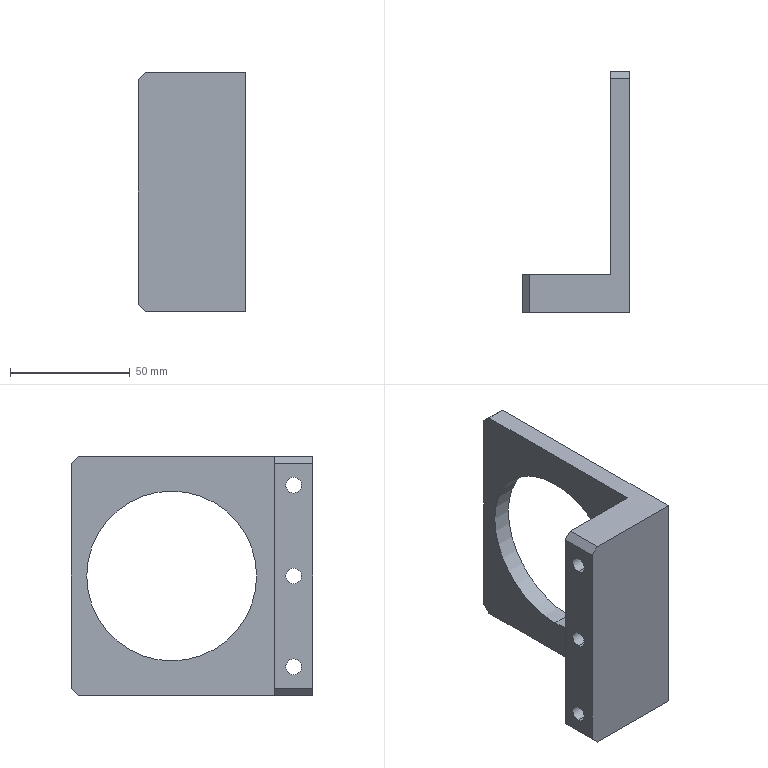Part | SolidWorks | features 3DProfileFeature 1, Chamfer 1, Extrusion 1, HoleWzd 1, ICE 1 | 1 solid | 29 faces | box 45 x 101 x 100 mm | volume 97106 mm3 | plane 15 | cylinder 14 | commonest cylinder face diameters 6.6 x6 11 x6 71 x2
STEP:
#1=CARTESIAN_POINT('',(-35.,8.,9.121));
#2=VERTEX_POINT('',#1);
#3=CARTESIAN_POINT('',(-35.,8.,-1.879));
#4=VERTEX_POINT('',#3);
#5=CARTESIAN_POINT('',(-35.,8.,3.621));
#6=DIRECTION('',(1.,0.,0.));
#7=DIRECTION('',(0.,0.,-1.));
#8=AXIS2_PLACEMENT_3D('',#5,#6,#7);
#9=CIRCLE('',#8,5.5);
#10=EDGE_CURVE('',#2,#4,#9,.T.);
#11=ORIENTED_EDGE('',*,*,#10,.F.);
#12=CARTESIAN_POINT('',(0.,8.,9.121));
#13=VERTEX_POINT('',#12);
#14=CARTESIAN_POINT('',(0.,8.,9.121));
#15=DIRECTION('',(1.,0.,0.));
#16=VECTOR('',#15,1000.);
#17=LINE('',#14,#16);
#18=EDGE_CURVE('',#2,#13,#17,.T.);
#19=ORIENTED_EDGE('',*,*,#18,.T.);
#20=CARTESIAN_POINT('',(0.,8.,-1.879));
#21=VERTEX_POINT('',#20);
#22=CARTESIAN_POINT('',(0.,8.,3.621));
#23=DIRECTION('',(1.,0.,0.));
#24=DIRECTION('',(0.,0.,-1.));
#25=AXIS2_PLACEMENT_3D('',#22,#23,#24);
#26=CIRCLE('',#25,5.5);
#27=EDGE_CURVE('',#13,#21,#26,.T.);
#28=ORIENTED_EDGE('',*,*,#27,.T.);
#29=CARTESIAN_POINT('',(0.,8.,-1.879));
#30=DIRECTION('',(1.,0.,0.));
#31=VECTOR('',#30,1000.);
#32=LINE('',#29,#31);
#33=EDGE_CURVE('',#4,#21,#32,.T.);
#34=ORIENTED_EDGE('',*,*,#33,.F.);
#35=EDGE_LOOP('',(#11,#19,#28,#34));
#36=FACE_OUTER_BOUND('',#35,.T.);
#37=CARTESIAN_POINT('',(0.,8.,3.621));
#38=DIRECTION('',(1.,0.,0.));
#39=DIRECTION('',(0.,0.,-1.));
#40=AXIS2_PLACEMENT_3D('',#37,#38,#39);
#41=CYLINDRICAL_SURFACE('',#40,5.5);
#42=ADVANCED_FACE('',(#36),#41,.F.);
#43=CARTESIAN_POINT('',(-45.,8.,6.921));
#44=VERTEX_POINT('',#43);
#45=CARTESIAN_POINT('',(-45.,8.,0.3205));
#46=VERTEX_POINT('',#45);
#47=CARTESIAN_POINT('',(-45.,8.,3.621));
#48=DIRECTION('',(1.,0.,0.));
#49=DIRECTION('',(0.,0.,-1.));
#50=AXIS2_PLACEMENT_3D('',#47,#48,#49);
#51=CIRCLE('',#50,3.3);
#52=EDGE_CURVE('',#44,#46,#51,.T.);
#53=ORIENTED_EDGE('',*,*,#52,.F.);
#54=CARTESIAN_POINT('',(-35.,8.,6.921));
#55=VERTEX_POINT('',#54);
#56=CARTESIAN_POINT('',(0.,8.,6.921));
#57=DIRECTION('',(1.,0.,0.));
#58=VECTOR('',#57,1000.);
#59=LINE('',#56,#58);
#60=EDGE_CURVE('',#44,#55,#59,.T.);
#61=ORIENTED_EDGE('',*,*,#60,.T.);
#62=CARTESIAN_POINT('',(-35.,8.,0.3205));
#63=VERTEX_POINT('',#62);
#64=CARTESIAN_POINT('',(-35.,8.,3.621));
#65=DIRECTION('',(1.,0.,0.));
#66=DIRECTION('',(0.,0.,-1.));
#67=AXIS2_PLACEMENT_3D('',#64,#65,#66);
#68=CIRCLE('',#67,3.3);
#69=EDGE_CURVE('',#55,#63,#68,.T.);
#70=ORIENTED_EDGE('',*,*,#69,.T.);
#71=CARTESIAN_POINT('',(0.,8.,0.3205));
#72=DIRECTION('',(1.,0.,0.));
#73=VECTOR('',#72,1000.);
#74=LINE('',#71,#73);
#75=EDGE_CURVE('',#46,#63,#74,.T.);
#76=ORIENTED_EDGE('',*,*,#75,.F.);
#77=EDGE_LOOP('',(#53,#61,#70,#76));
#78=FACE_OUTER_BOUND('',#77,.T.);
#79=CARTESIAN_POINT('',(0.,8.,3.621));
#80=DIRECTION('',(1.,0.,0.));
#81=DIRECTION('',(0.,0.,-1.));
#82=AXIS2_PLACEMENT_3D('',#79,#80,#81);
#83=CYLINDRICAL_SURFACE('',#82,3.3);
#84=ADVANCED_FACE('',(#78),#83,.F.);
#85=CARTESIAN_POINT('',(-35.,8.,-28.879));
#86=VERTEX_POINT('',#85);
#87=CARTESIAN_POINT('',(-35.,8.,-39.879));
#88=VERTEX_POINT('',#87);
#89=CARTESIAN_POINT('',(-35.,8.,-34.379));
#90=DIRECTION('',(1.,0.,0.));
#91=DIRECTION('',(0.,0.,-1.));
#92=AXIS2_PLACEMENT_3D('',#89,#90,#91);
#93=CIRCLE('',#92,5.5);
#94=EDGE_CURVE('',#86,#88,#93,.T.);
#95=ORIENTED_EDGE('',*,*,#94,.F.);
#96=CARTESIAN_POINT('',(0.,8.,-28.879));
#97=VERTEX_POINT('',#96);
#98=CARTESIAN_POINT('',(0.,8.,-28.879));
#99=DIRECTION('',(1.,0.,0.));
#100=VECTOR('',#99,1000.);
#101=LINE('',#98,#100);
#102=EDGE_CURVE('',#86,#97,#101,.T.);
#103=ORIENTED_EDGE('',*,*,#102,.T.);
#104=CARTESIAN_POINT('',(0.,8.,-39.879));
#105=VERTEX_POINT('',#104);
#106=CARTESIAN_POINT('',(0.,8.,-34.379));
#107=DIRECTION('',(1.,0.,0.));
#108=DIRECTION('',(0.,0.,-1.));
#109=AXIS2_PLACEMENT_3D('',#106,#107,#108);
#110=CIRCLE('',#109,5.5);
#111=EDGE_CURVE('',#97,#105,#110,.T.);
#112=ORIENTED_EDGE('',*,*,#111,.T.);
#113=CARTESIAN_POINT('',(0.,8.,-39.879));
#114=DIRECTION('',(1.,0.,0.));
#115=VECTOR('',#114,1000.);
#116=LINE('',#113,#115);
#117=EDGE_CURVE('',#88,#105,#116,.T.);
#118=ORIENTED_EDGE('',*,*,#117,.F.);
#119=EDGE_LOOP('',(#95,#103,#112,#118));
#120=FACE_OUTER_BOUND('',#119,.T.);
#121=CARTESIAN_POINT('',(0.,8.,-34.379));
#122=DIRECTION('',(1.,0.,0.));
#123=DIRECTION('',(0.,0.,-1.));
#124=AXIS2_PLACEMENT_3D('',#121,#122,#123);
#125=CYLINDRICAL_SURFACE('',#124,5.5);
#126=ADVANCED_FACE('',(#120),#125,.F.);
#127=CARTESIAN_POINT('',(-45.,8.,-31.079));
#128=VERTEX_POINT('',#127);
#129=CARTESIAN_POINT('',(-45.,8.,-37.679));
#130=VERTEX_POINT('',#129);
#131=CARTESIAN_POINT('',(-45.,8.,-34.379));
#132=DIRECTION('',(1.,0.,0.));
#133=DIRECTION('',(0.,0.,-1.));
#134=AXIS2_PLACEMENT_3D('',#131,#132,#133);
#135=CIRCLE('',#134,3.3);
#136=EDGE_CURVE('',#128,#130,#135,.T.);
#137=ORIENTED_EDGE('',*,*,#136,.F.);
#138=CARTESIAN_POINT('',(-35.,8.,-31.079));
#139=VERTEX_POINT('',#138);
#140=CARTESIAN_POINT('',(0.,8.,-31.079));
#141=DIRECTION('',(1.,0.,0.));
#142=VECTOR('',#141,1000.);
#143=LINE('',#140,#142);
#144=EDGE_CURVE('',#128,#139,#143,.T.);
#145=ORIENTED_EDGE('',*,*,#144,.T.);
#146=CARTESIAN_POINT('',(-35.,8.,-37.679));
#147=VERTEX_POINT('',#146);
#148=CARTESIAN_POINT('',(-35.,8.,-34.379));
#149=DIRECTION('',(1.,0.,0.));
#150=DIRECTION('',(0.,0.,-1.));
#151=AXIS2_PLACEMENT_3D('',#148,#149,#150);
#152=CIRCLE('',#151,3.3);
#153=EDGE_CURVE('',#139,#147,#152,.T.);
#154=ORIENTED_EDGE('',*,*,#153,.T.);
#155=CARTESIAN_POINT('',(0.,8.,-37.679));
#156=DIRECTION('',(1.,0.,0.));
#157=VECTOR('',#156,1000.);
#158=LINE('',#155,#157);
#159=EDGE_CURVE('',#130,#147,#158,.T.);
#160=ORIENTED_EDGE('',*,*,#159,.F.);
#161=EDGE_LOOP('',(#137,#145,#154,#160));
#162=FACE_OUTER_BOUND('',#161,.T.);
#163=CARTESIAN_POINT('',(0.,8.,-34.379));
#164=DIRECTION('',(1.,0.,0.));
#165=DIRECTION('',(0.,0.,-1.));
#166=AXIS2_PLACEMENT_3D('',#163,#164,#165);
#167=CYLINDRICAL_SURFACE('',#166,3.3);
#168=ADVANCED_FACE('',(#162),#167,.F.);
#169=CARTESIAN_POINT('',(-35.,8.,-66.879));
#170=VERTEX_POINT('',#169);
#171=CARTESIAN_POINT('',(-35.,8.,-77.879));
#172=VERTEX_POINT('',#171);
#173=CARTESIAN_POINT('',(-35.,8.,-72.379));
#174=DIRECTION('',(1.,0.,0.));
#175=DIRECTION('',(0.,0.,-1.));
#176=AXIS2_PLACEMENT_3D('',#173,#174,#175);
#177=CIRCLE('',#176,5.5);
#178=EDGE_CURVE('',#170,#172,#177,.T.);
#179=ORIENTED_EDGE('',*,*,#178,.F.);
#180=CARTESIAN_POINT('',(0.,8.,-66.879));
#181=VERTEX_POINT('',#180);
#182=CARTESIAN_POINT('',(0.,8.,-66.879));
#183=DIRECTION('',(1.,0.,0.));
#184=VECTOR('',#183,1000.);
#185=LINE('',#182,#184);
#186=EDGE_CURVE('',#170,#181,#185,.T.);
#187=ORIENTED_EDGE('',*,*,#186,.T.);
#188=CARTESIAN_POINT('',(0.,8.,-77.879));
#189=VERTEX_POINT('',#188);
#190=CARTESIAN_POINT('',(0.,8.,-72.379));
#191=DIRECTION('',(1.,0.,0.));
#192=DIRECTION('',(0.,0.,-1.));
#193=AXIS2_PLACEMENT_3D('',#190,#191,#192);
#194=CIRCLE('',#193,5.5);
#195=EDGE_CURVE('',#181,#189,#194,.T.);
#196=ORIENTED_EDGE('',*,*,#195,.T.);
#197=CARTESIAN_POINT('',(0.,8.,-77.879));
#198=DIRECTION('',(1.,0.,0.));
#199=VECTOR('',#198,1000.);
#200=LINE('',#197,#199);
#201=EDGE_CURVE('',#172,#189,#200,.T.);
#202=ORIENTED_EDGE('',*,*,#201,.F.);
#203=EDGE_LOOP('',(#179,#187,#196,#202));
#204=FACE_OUTER_BOUND('',#203,.T.);
#205=CARTESIAN_POINT('',(0.,8.,-72.379));
#206=DIRECTION('',(1.,0.,0.));
#207=DIRECTION('',(0.,0.,-1.));
#208=AXIS2_PLACEMENT_3D('',#205,#206,#207);
#209=CYLINDRICAL_SURFACE('',#208,5.5);
#210=ADVANCED_FACE('',(#204),#209,.F.);
#211=CARTESIAN_POINT('',(-45.,8.,-69.079));
#212=VERTEX_POINT('',#211);
#213=CARTESIAN_POINT('',(-45.,8.,-75.679));
#214=VERTEX_POINT('',#213);
#215=CARTESIAN_POINT('',(-45.,8.,-72.379));
#216=DIRECTION('',(1.,0.,0.));
#217=DIRECTION('',(0.,0.,-1.));
#218=AXIS2_PLACEMENT_3D('',#215,#216,#217);
#219=CIRCLE('',#218,3.3);
#220=EDGE_CURVE('',#212,#214,#219,.T.);
#221=ORIENTED_EDGE('',*,*,#220,.F.);
#222=CARTESIAN_POINT('',(-35.,8.,-69.079));
#223=VERTEX_POINT('',#222);
#224=CARTESIAN_POINT('',(0.,8.,-69.079));
#225=DIRECTION('',(1.,0.,0.));
#226=VECTOR('',#225,1000.);
#227=LINE('',#224,#226);
#228=EDGE_CURVE('',#212,#223,#227,.T.);
#229=ORIENTED_EDGE('',*,*,#228,.T.);
#230=CARTESIAN_POINT('',(-35.,8.,-75.679));
#231=VERTEX_POINT('',#230);
#232=CARTESIAN_POINT('',(-35.,8.,-72.379));
#233=DIRECTION('',(1.,0.,0.));
#234=DIRECTION('',(0.,0.,-1.));
#235=AXIS2_PLACEMENT_3D('',#232,#233,#234);
#236=CIRCLE('',#235,3.3);
#237=EDGE_CURVE('',#223,#231,#236,.T.);
#238=ORIENTED_EDGE('',*,*,#237,.T.);
#239=CARTESIAN_POINT('',(0.,8.,-75.679));
#240=DIRECTION('',(1.,0.,0.));
#241=VECTOR('',#240,1000.);
#242=LINE('',#239,#241);
#243=EDGE_CURVE('',#214,#231,#242,.T.);
#244=ORIENTED_EDGE('',*,*,#243,.F.);
#245=EDGE_LOOP('',(#221,#229,#238,#244));
#246=FACE_OUTER_BOUND('',#245,.T.);
#247=CARTESIAN_POINT('',(0.,8.,-72.379));
#248=DIRECTION('',(1.,0.,0.));
#249=DIRECTION('',(0.,0.,-1.));
#250=AXIS2_PLACEMENT_3D('',#247,#248,#249);
#251=CYLINDRICAL_SURFACE('',#250,3.3);
#252=ADVANCED_FACE('',(#246),#251,.F.);
#253=CARTESIAN_POINT('',(0.,59.,1.121));
#254=VERTEX_POINT('',#253);
#255=CARTESIAN_POINT('',(0.,59.,-69.879));
#256=VERTEX_POINT('',#255);
#257=CARTESIAN_POINT('',(0.,59.,-34.379));
#258=DIRECTION('',(1.,0.,0.));
#259=DIRECTION('',(0.,0.,1.));
#260=AXIS2_PLACEMENT_3D('',#257,#258,#259);
#261=CIRCLE('',#260,35.5);
#262=EDGE_CURVE('',#254,#256,#261,.T.);
#263=ORIENTED_EDGE('',*,*,#262,.T.);
#264=CARTESIAN_POINT('',(-8.,59.,-69.879));
#265=VERTEX_POINT('',#264);
#266=CARTESIAN_POINT('',(0.001,59.,-69.879));
#267=DIRECTION('',(-1.,0.,0.));
#268=VECTOR('',#267,1000.);
#269=LINE('',#266,#268);
#270=EDGE_CURVE('',#256,#265,#269,.T.);
#271=ORIENTED_EDGE('',*,*,#270,.T.);
#272=CARTESIAN_POINT('',(-8.,59.,1.121));
#273=VERTEX_POINT('',#272);
#274=CARTESIAN_POINT('',(-8.,59.,-34.379));
#275=DIRECTION('',(-1.,0.,0.));
#276=DIRECTION('',(0.,0.,1.));
#277=AXIS2_PLACEMENT_3D('',#274,#275,#276);
#278=CIRCLE('',#277,35.5);
#279=EDGE_CURVE('',#265,#273,#278,.T.);
#280=ORIENTED_EDGE('',*,*,#279,.T.);
#281=CARTESIAN_POINT('',(0.001,59.,1.121));
#282=DIRECTION('',(-1.,0.,0.));
#283=VECTOR('',#282,1000.);
#284=LINE('',#281,#283);
#285=EDGE_CURVE('',#254,#273,#284,.T.);
#286=ORIENTED_EDGE('',*,*,#285,.F.);
#287=EDGE_LOOP('',(#263,#271,#280,#286));
#288=FACE_OUTER_BOUND('',#287,.T.);
#289=CARTESIAN_POINT('',(0.001,59.,-34.379));
#290=DIRECTION('',(-1.,0.,0.));
#291=DIRECTION('',(0.,0.,1.));
#292=AXIS2_PLACEMENT_3D('',#289,#290,#291);
#293=CYLINDRICAL_SURFACE('',#292,35.5);
#294=ADVANCED_FACE('',(#288),#293,.F.);
#295=CARTESIAN_POINT('',(0.,8.,-34.379));
#296=DIRECTION('',(1.,0.,0.));
#297=DIRECTION('',(0.,0.,-1.));
#298=AXIS2_PLACEMENT_3D('',#295,#296,#297);
#299=CIRCLE('',#298,5.5);
#300=EDGE_CURVE('',#105,#97,#299,.T.);
#301=ORIENTED_EDGE('',*,*,#300,.F.);
#302=ORIENTED_EDGE('',*,*,#111,.F.);
#303=EDGE_LOOP('',(#301,#302));
#304=FACE_BOUND('',#303,.T.);
#305=ORIENTED_EDGE('',*,*,#262,.F.);
#306=CARTESIAN_POINT('',(0.,59.,-34.379));
#307=DIRECTION('',(1.,0.,0.));
#308=DIRECTION('',(0.,0.,1.));
#309=AXIS2_PLACEMENT_3D('',#306,#307,#308);
#310=CIRCLE('',#309,35.5);
#311=EDGE_CURVE('',#256,#254,#310,.T.);
#312=ORIENTED_EDGE('',*,*,#311,.F.);
#313=EDGE_LOOP('',(#305,#312));
#314=FACE_BOUND('',#313,.T.);
#315=CARTESIAN_POINT('',(0.,101.,12.621));
#316=VERTEX_POINT('',#315);
#317=CARTESIAN_POINT('',(0.,101.,-81.379));
#318=VERTEX_POINT('',#317);
#319=CARTESIAN_POINT('',(0.,101.,15.621));
#320=DIRECTION('',(0.,0.,-1.));
#321=VECTOR('',#320,1000.);
#322=LINE('',#319,#321);
#323=EDGE_CURVE('',#316,#318,#322,.T.);
#324=ORIENTED_EDGE('',*,*,#323,.F.);
#325=CARTESIAN_POINT('',(0.,98.,15.621));
#326=VERTEX_POINT('',#325);
#327=CARTESIAN_POINT('',(0.,98.,15.621));
#328=DIRECTION('',(0.,-0.7071,0.7071));
#329=VECTOR('',#328,1000.);
#330=LINE('',#327,#329);
#331=EDGE_CURVE('',#316,#326,#330,.T.);
#332=ORIENTED_EDGE('',*,*,#331,.T.);
#333=CARTESIAN_POINT('',(0.,0.,15.621));
#334=VERTEX_POINT('',#333);
#335=CARTESIAN_POINT('',(0.,101.,15.621));
#336=DIRECTION('',(0.,1.,0.));
#337=VECTOR('',#336,1000.);
#338=LINE('',#335,#337);
#339=EDGE_CURVE('',#334,#326,#338,.T.);
#340=ORIENTED_EDGE('',*,*,#339,.F.);
#341=CARTESIAN_POINT('',(0.,0.,-84.379));
#342=VERTEX_POINT('',#341);
#343=CARTESIAN_POINT('',(0.,0.,15.621));
#344=DIRECTION('',(0.,0.,-1.));
#345=VECTOR('',#344,1000.);
#346=LINE('',#343,#345);
#347=EDGE_CURVE('',#334,#342,#346,.T.);
#348=ORIENTED_EDGE('',*,*,#347,.T.);
#349=CARTESIAN_POINT('',(0.,98.,-84.379));
#350=VERTEX_POINT('',#349);
#351=CARTESIAN_POINT('',(0.,101.,-84.379));
#352=DIRECTION('',(0.,1.,0.));
#353=VECTOR('',#352,1000.);
#354=LINE('',#351,#353);
#355=EDGE_CURVE('',#342,#350,#354,.T.);
#356=ORIENTED_EDGE('',*,*,#355,.T.);
#357=CARTESIAN_POINT('',(0.,101.,-81.379));
#358=DIRECTION('',(0.,0.7071,0.7071));
#359=VECTOR('',#358,1000.);
#360=LINE('',#357,#359);
#361=EDGE_CURVE('',#350,#318,#360,.T.);
#362=ORIENTED_EDGE('',*,*,#361,.T.);
#363=EDGE_LOOP('',(#324,#332,#340,#348,#356,#362));
#364=FACE_OUTER_BOUND('',#363,.T.);
#365=CARTESIAN_POINT('',(0.,8.,-72.379));
#366=DIRECTION('',(1.,0.,0.));
#367=DIRECTION('',(0.,0.,-1.));
#368=AXIS2_PLACEMENT_3D('',#365,#366,#367);
#369=CIRCLE('',#368,5.5);
#370=EDGE_CURVE('',#189,#181,#369,.T.);
#371=ORIENTED_EDGE('',*,*,#370,.F.);
#372=ORIENTED_EDGE('',*,*,#195,.F.);
#373=EDGE_LOOP('',(#371,#372));
#374=FACE_BOUND('',#373,.T.);
#375=CARTESIAN_POINT('',(0.,8.,3.621));
#376=DIRECTION('',(1.,0.,0.));
#377=DIRECTION('',(0.,0.,-1.));
#378=AXIS2_PLACEMENT_3D('',#375,#376,#377);
#379=CIRCLE('',#378,5.5);
#380=EDGE_CURVE('',#21,#13,#379,.T.);
#381=ORIENTED_EDGE('',*,*,#380,.F.);
#382=ORIENTED_EDGE('',*,*,#27,.F.);
#383=EDGE_LOOP('',(#381,#382));
#384=FACE_BOUND('',#383,.T.);
#385=CARTESIAN_POINT('',(0.,101.,15.621));
#386=DIRECTION('',(-1.,0.,0.));
#387=DIRECTION('',(0.,0.,1.));
#388=AXIS2_PLACEMENT_3D('',#385,#386,#387);
#389=PLANE('',#388);
#390=ADVANCED_FACE('',(#304,#314,#364,#374,#384),#389,.F.);
#391=CARTESIAN_POINT('',(-8.,101.,12.621));
#392=VERTEX_POINT('',#391);
#393=CARTESIAN_POINT('',(-8.,101.,-81.379));
#394=VERTEX_POINT('',#393);
#395=CARTESIAN_POINT('',(-8.,101.,15.621));
#396=DIRECTION('',(0.,0.,-1.));
#397=VECTOR('',#396,1000.);
#398=LINE('',#395,#397);
#399=EDGE_CURVE('',#392,#394,#398,.T.);
#400=ORIENTED_EDGE('',*,*,#399,.F.);
#401=CARTESIAN_POINT('',(-8.,101.,12.621));
#402=DIRECTION('',(1.,0.,0.));
#403=VECTOR('',#402,1000.);
#404=LINE('',#401,#403);
#405=EDGE_CURVE('',#392,#316,#404,.T.);
#406=ORIENTED_EDGE('',*,*,#405,.T.);
#407=ORIENTED_EDGE('',*,*,#323,.T.);
#408=CARTESIAN_POINT('',(-8.,101.,-81.379));
#409=DIRECTION('',(-1.,0.,0.));
#410=VECTOR('',#409,1000.);
#411=LINE('',#408,#410);
#412=EDGE_CURVE('',#318,#394,#411,.T.);
#413=ORIENTED_EDGE('',*,*,#412,.T.);
#414=EDGE_LOOP('',(#400,#406,#407,#413));
#415=FACE_OUTER_BOUND('',#414,.T.);
#416=CARTESIAN_POINT('',(-8.,101.,15.621));
#417=DIRECTION('',(0.,-1.,0.));
#418=DIRECTION('',(0.,0.,-1.));
#419=AXIS2_PLACEMENT_3D('',#416,#417,#418);
#420=PLANE('',#419);
#421=ADVANCED_FACE('',(#415),#420,.F.);
#422=CARTESIAN_POINT('',(-8.,59.,-34.379));
#423=DIRECTION('',(-1.,0.,0.));
#424=DIRECTION('',(0.,0.,1.));
#425=AXIS2_PLACEMENT_3D('',#422,#423,#424);
#426=CIRCLE('',#425,35.5);
#427=EDGE_CURVE('',#273,#265,#426,.T.);
#428=ORIENTED_EDGE('',*,*,#427,.F.);
#429=ORIENTED_EDGE('',*,*,#279,.F.);
#430=EDGE_LOOP('',(#428,#429));
#431=FACE_BOUND('',#430,.T.);
#432=CARTESIAN_POINT('',(-8.,98.,15.621));
#433=VERTEX_POINT('',#432);
#434=CARTESIAN_POINT('',(-8.,16.,15.621));
#435=VERTEX_POINT('',#434);
#436=CARTESIAN_POINT('',(-8.,16.,15.621));
#437=DIRECTION('',(0.,-1.,0.));
#438=VECTOR('',#437,1000.);
#439=LINE('',#436,#438);
#440=EDGE_CURVE('',#433,#435,#439,.T.);
#441=ORIENTED_EDGE('',*,*,#440,.F.);
#442=CARTESIAN_POINT('',(-8.,98.,15.621));
#443=DIRECTION('',(0.,0.7071,-0.7071));
#444=VECTOR('',#443,1000.);
#445=LINE('',#442,#444);
#446=EDGE_CURVE('',#433,#392,#445,.T.);
#447=ORIENTED_EDGE('',*,*,#446,.T.);
#448=ORIENTED_EDGE('',*,*,#399,.T.);
#449=CARTESIAN_POINT('',(-8.,98.,-84.379));
#450=VERTEX_POINT('',#449);
#451=CARTESIAN_POINT('',(-8.,101.,-81.379));
#452=DIRECTION('',(0.,-0.7071,-0.7071));
#453=VECTOR('',#452,1000.);
#454=LINE('',#451,#453);
#455=EDGE_CURVE('',#394,#450,#454,.T.);
#456=ORIENTED_EDGE('',*,*,#455,.T.);
#457=CARTESIAN_POINT('',(-8.,16.,-84.379));
#458=VERTEX_POINT('',#457);
#459=CARTESIAN_POINT('',(-8.,16.,-84.379));
#460=DIRECTION('',(0.,-1.,0.));
#461=VECTOR('',#460,1000.);
#462=LINE('',#459,#461);
#463=EDGE_CURVE('',#450,#458,#462,.T.);
#464=ORIENTED_EDGE('',*,*,#463,.T.);
#465=CARTESIAN_POINT('',(-8.,16.,15.621));
#466=DIRECTION('',(0.,0.,-1.));
#467=VECTOR('',#466,1000.);
#468=LINE('',#465,#467);
#469=EDGE_CURVE('',#435,#458,#468,.T.);
#470=ORIENTED_EDGE('',*,*,#469,.F.);
#471=EDGE_LOOP('',(#441,#447,#448,#456,#464,#470));
#472=FACE_OUTER_BOUND('',#471,.T.);
#473=CARTESIAN_POINT('',(-8.,16.,15.621));
#474=DIRECTION('',(1.,0.,0.));
#475=DIRECTION('',(0.,0.,-1.));
#476=AXIS2_PLACEMENT_3D('',#473,#474,#475);
#477=PLANE('',#476);
#478=ADVANCED_FACE('',(#431,#472),#477,.F.);
#479=CARTESIAN_POINT('',(-42.,16.,-84.379));
#480=VERTEX_POINT('',#479);
#481=CARTESIAN_POINT('',(-45.,16.,-84.379));
#482=DIRECTION('',(-1.,0.,0.));
#483=VECTOR('',#482,1000.);
#484=LINE('',#481,#483);
#485=EDGE_CURVE('',#458,#480,#484,.T.);
#486=ORIENTED_EDGE('',*,*,#485,.T.);
#487=CARTESIAN_POINT('',(-45.,16.,-81.379));
#488=VERTEX_POINT('',#487);
#489=CARTESIAN_POINT('',(-45.,16.,-81.379));
#490=DIRECTION('',(-0.7071,0.,0.7071));
#491=VECTOR('',#490,1000.);
#492=LINE('',#489,#491);
#493=EDGE_CURVE('',#480,#488,#492,.T.);
#494=ORIENTED_EDGE('',*,*,#493,.T.);
#495=CARTESIAN_POINT('',(-45.,16.,12.621));
#496=VERTEX_POINT('',#495);
#497=CARTESIAN_POINT('',(-45.,16.,15.621));
#498=DIRECTION('',(0.,0.,-1.));
#499=VECTOR('',#498,1000.);
#500=LINE('',#497,#499);
#501=EDGE_CURVE('',#496,#488,#500,.T.);
#502=ORIENTED_EDGE('',*,*,#501,.F.);
#503=CARTESIAN_POINT('',(-42.,16.,15.621));
#504=VERTEX_POINT('',#503);
#505=CARTESIAN_POINT('',(-42.,16.,15.621));
#506=DIRECTION('',(0.7071,0.,0.7071));
#507=VECTOR('',#506,1000.);
#508=LINE('',#505,#507);
#509=EDGE_CURVE('',#496,#504,#508,.T.);
#510=ORIENTED_EDGE('',*,*,#509,.T.);
#511=CARTESIAN_POINT('',(-45.,16.,15.621));
#512=DIRECTION('',(-1.,0.,0.));
#513=VECTOR('',#512,1000.);
#514=LINE('',#511,#513);
#515=EDGE_CURVE('',#435,#504,#514,.T.);
#516=ORIENTED_EDGE('',*,*,#515,.F.);
#517=ORIENTED_EDGE('',*,*,#469,.T.);
#518=EDGE_LOOP('',(#486,#494,#502,#510,#516,#517));
#519=FACE_OUTER_BOUND('',#518,.T.);
#520=CARTESIAN_POINT('',(-45.,16.,15.621));
#521=DIRECTION('',(0.,-1.,0.));
#522=DIRECTION('',(1.,0.,0.));
#523=AXIS2_PLACEMENT_3D('',#520,#521,#522);
#524=PLANE('',#523);
#525=ADVANCED_FACE('',(#519),#524,.F.);
#526=CARTESIAN_POINT('',(-45.,8.,3.621));
#527=DIRECTION('',(1.,0.,0.));
#528=DIRECTION('',(0.,0.,-1.));
#529=AXIS2_PLACEMENT_3D('',#526,#527,#528);
#530=CIRCLE('',#529,3.3);
#531=EDGE_CURVE('',#46,#44,#530,.T.);
#532=ORIENTED_EDGE('',*,*,#531,.T.);
#533=ORIENTED_EDGE('',*,*,#52,.T.);
#534=EDGE_LOOP('',(#532,#533));
#535=FACE_BOUND('',#534,.T.);
#536=CARTESIAN_POINT('',(-45.,8.,-34.379));
#537=DIRECTION('',(1.,0.,0.));
#538=DIRECTION('',(0.,0.,-1.));
#539=AXIS2_PLACEMENT_3D('',#536,#537,#538);
#540=CIRCLE('',#539,3.3);
#541=EDGE_CURVE('',#130,#128,#540,.T.);
#542=ORIENTED_EDGE('',*,*,#541,.T.);
#543=ORIENTED_EDGE('',*,*,#136,.T.);
#544=EDGE_LOOP('',(#542,#543));
#545=FACE_BOUND('',#544,.T.);
#546=CARTESIAN_POINT('',(-45.,8.,-72.379));
#547=DIRECTION('',(1.,0.,0.));
#548=DIRECTION('',(0.,0.,-1.));
#549=AXIS2_PLACEMENT_3D('',#546,#547,#548);
#550=CIRCLE('',#549,3.3);
#551=EDGE_CURVE('',#214,#212,#550,.T.);
#552=ORIENTED_EDGE('',*,*,#551,.T.);
#553=ORIENTED_EDGE('',*,*,#220,.T.);
#554=EDGE_LOOP('',(#552,#553));
#555=FACE_BOUND('',#554,.T.);
#556=ORIENTED_EDGE('',*,*,#501,.T.);
#557=CARTESIAN_POINT('',(-45.,0.,-81.379));
#558=VERTEX_POINT('',#557);
#559=CARTESIAN_POINT('',(-45.,0.,-81.379));
#560=DIRECTION('',(0.,-1.,0.));
#561=VECTOR('',#560,1000.);
#562=LINE('',#559,#561);
#563=EDGE_CURVE('',#488,#558,#562,.T.);
#564=ORIENTED_EDGE('',*,*,#563,.T.);
#565=CARTESIAN_POINT('',(-45.,0.,12.621));
#566=VERTEX_POINT('',#565);
#567=CARTESIAN_POINT('',(-45.,0.,15.621));
#568=DIRECTION('',(0.,0.,-1.));
#569=VECTOR('',#568,1000.);
#570=LINE('',#567,#569);
#571=EDGE_CURVE('',#566,#558,#570,.T.);
#572=ORIENTED_EDGE('',*,*,#571,.F.);
#573=CARTESIAN_POINT('',(-45.,0.,12.621));
#574=DIRECTION('',(0.,1.,0.));
#575=VECTOR('',#574,1000.);
#576=LINE('',#573,#575);
#577=EDGE_CURVE('',#566,#496,#576,.T.);
#578=ORIENTED_EDGE('',*,*,#577,.T.);
#579=EDGE_LOOP('',(#556,#564,#572,#578));
#580=FACE_OUTER_BOUND('',#579,.T.);
#581=CARTESIAN_POINT('',(-45.,0.,15.621));
#582=DIRECTION('',(1.,0.,0.));
#583=DIRECTION('',(0.,0.,-1.));
#584=AXIS2_PLACEMENT_3D('',#581,#582,#583);
#585=PLANE('',#584);
#586=ADVANCED_FACE('',(#535,#545,#555,#580),#585,.F.);
#587=ORIENTED_EDGE('',*,*,#571,.T.);
#588=CARTESIAN_POINT('',(-42.,0.,-84.379));
#589=VERTEX_POINT('',#588);
#590=CARTESIAN_POINT('',(-45.,0.,-81.379));
#591=DIRECTION('',(0.7071,0.,-0.7071));
#592=VECTOR('',#591,1000.);
#593=LINE('',#590,#592);
#594=EDGE_CURVE('',#558,#589,#593,.T.);
#595=ORIENTED_EDGE('',*,*,#594,.T.);
#596=CARTESIAN_POINT('',(0.,0.,-84.379));
#597=DIRECTION('',(1.,0.,0.));
#598=VECTOR('',#597,1000.);
#599=LINE('',#596,#598);
#600=EDGE_CURVE('',#589,#342,#599,.T.);
#601=ORIENTED_EDGE('',*,*,#600,.T.);
#602=ORIENTED_EDGE('',*,*,#347,.F.);
#603=CARTESIAN_POINT('',(-42.,0.,15.621));
#604=VERTEX_POINT('',#603);
#605=CARTESIAN_POINT('',(0.,0.,15.621));
#606=DIRECTION('',(1.,0.,0.));
#607=VECTOR('',#606,1000.);
#608=LINE('',#605,#607);
#609=EDGE_CURVE('',#604,#334,#608,.T.);
#610=ORIENTED_EDGE('',*,*,#609,.F.);
#611=CARTESIAN_POINT('',(-42.,0.,15.621));
#612=DIRECTION('',(-0.7071,0.,-0.7071));
#613=VECTOR('',#612,1000.);
#614=LINE('',#611,#613);
#615=EDGE_CURVE('',#604,#566,#614,.T.);
#616=ORIENTED_EDGE('',*,*,#615,.T.);
#617=EDGE_LOOP('',(#587,#595,#601,#602,#610,#616));
#618=FACE_OUTER_BOUND('',#617,.T.);
#619=CARTESIAN_POINT('',(0.,0.,15.621));
#620=DIRECTION('',(0.,1.,0.));
#621=DIRECTION('',(-1.,0.,0.));
#622=AXIS2_PLACEMENT_3D('',#619,#620,#621);
#623=PLANE('',#622);
#624=ADVANCED_FACE('',(#618),#623,.F.);
#625=ORIENTED_EDGE('',*,*,#515,.T.);
#626=CARTESIAN_POINT('',(-42.,0.,15.621));
#627=DIRECTION('',(0.,-1.,0.));
#628=VECTOR('',#627,1000.);
#629=LINE('',#626,#628);
#630=EDGE_CURVE('',#504,#604,#629,.T.);
#631=ORIENTED_EDGE('',*,*,#630,.T.);
#632=ORIENTED_EDGE('',*,*,#609,.T.);
#633=ORIENTED_EDGE('',*,*,#339,.T.);
#634=CARTESIAN_POINT('',(0.,98.,15.621));
#635=DIRECTION('',(-1.,0.,0.));
#636=VECTOR('',#635,1000.);
#637=LINE('',#634,#636);
#638=EDGE_CURVE('',#326,#433,#637,.T.);
#639=ORIENTED_EDGE('',*,*,#638,.T.);
#640=ORIENTED_EDGE('',*,*,#440,.T.);
#641=EDGE_LOOP('',(#625,#631,#632,#633,#639,#640));
#642=FACE_OUTER_BOUND('',#641,.T.);
#643=CARTESIAN_POINT('',(0.,0.,15.621));
#644=DIRECTION('',(0.,0.,-1.));
#645=DIRECTION('',(-1.,0.,0.));
#646=AXIS2_PLACEMENT_3D('',#643,#644,#645);
#647=PLANE('',#646);
#648=ADVANCED_FACE('',(#642),#647,.F.);
#649=ORIENTED_EDGE('',*,*,#600,.F.);
#650=CARTESIAN_POINT('',(-42.,16.,-84.379));
#651=DIRECTION('',(0.,1.,0.));
#652=VECTOR('',#651,1000.);
#653=LINE('',#650,#652);
#654=EDGE_CURVE('',#589,#480,#653,.T.);
#655=ORIENTED_EDGE('',*,*,#654,.T.);
#656=ORIENTED_EDGE('',*,*,#485,.F.);
#657=ORIENTED_EDGE('',*,*,#463,.F.);
#658=CARTESIAN_POINT('',(0.,98.,-84.379));
#659=DIRECTION('',(1.,0.,0.));
#660=VECTOR('',#659,1000.);
#661=LINE('',#658,#660);
#662=EDGE_CURVE('',#450,#350,#661,.T.);
#663=ORIENTED_EDGE('',*,*,#662,.T.);
#664=ORIENTED_EDGE('',*,*,#355,.F.);
#665=EDGE_LOOP('',(#649,#655,#656,#657,#663,#664));
#666=FACE_OUTER_BOUND('',#665,.T.);
#667=CARTESIAN_POINT('',(0.,0.,-84.379));
#668=DIRECTION('',(0.,0.,-1.));
#669=DIRECTION('',(-1.,0.,0.));
#670=AXIS2_PLACEMENT_3D('',#667,#668,#669);
#671=PLANE('',#670);
#672=ADVANCED_FACE('',(#666),#671,.T.);
#673=ORIENTED_EDGE('',*,*,#493,.F.);
#674=ORIENTED_EDGE('',*,*,#654,.F.);
#675=ORIENTED_EDGE('',*,*,#594,.F.);
#676=ORIENTED_EDGE('',*,*,#563,.F.);
#677=EDGE_LOOP('',(#673,#674,#675,#676));
#678=FACE_OUTER_BOUND('',#677,.T.);
#679=CARTESIAN_POINT('',(-45.,0.,-81.379));
#680=DIRECTION('',(-0.7071,0.,-0.7071));
#681=DIRECTION('',(0.,1.,0.));
#682=AXIS2_PLACEMENT_3D('',#679,#680,#681);
#683=PLANE('',#682);
#684=ADVANCED_FACE('',(#678),#683,.T.);
#685=ORIENTED_EDGE('',*,*,#509,.F.);
#686=ORIENTED_EDGE('',*,*,#577,.F.);
#687=ORIENTED_EDGE('',*,*,#615,.F.);
#688=ORIENTED_EDGE('',*,*,#630,.F.);
#689=EDGE_LOOP('',(#685,#686,#687,#688));
#690=FACE_OUTER_BOUND('',#689,.T.);
#691=CARTESIAN_POINT('',(-42.,0.,15.621));
#692=DIRECTION('',(0.7071,0.,-0.7071));
#693=DIRECTION('',(0.,-1.,0.));
#694=AXIS2_PLACEMENT_3D('',#691,#692,#693);
#695=PLANE('',#694);
#696=ADVANCED_FACE('',(#690),#695,.F.);
#697=ORIENTED_EDGE('',*,*,#331,.F.);
#698=ORIENTED_EDGE('',*,*,#405,.F.);
#699=ORIENTED_EDGE('',*,*,#446,.F.);
#700=ORIENTED_EDGE('',*,*,#638,.F.);
#701=EDGE_LOOP('',(#697,#698,#699,#700));
#702=FACE_OUTER_BOUND('',#701,.T.);
#703=CARTESIAN_POINT('',(0.,98.,15.621));
#704=DIRECTION('',(0.,-0.7071,-0.7071));
#705=DIRECTION('',(-1.,0.,0.));
#706=AXIS2_PLACEMENT_3D('',#703,#704,#705);
#707=PLANE('',#706);
#708=ADVANCED_FACE('',(#702),#707,.F.);
#709=ORIENTED_EDGE('',*,*,#361,.F.);
#710=ORIENTED_EDGE('',*,*,#662,.F.);
#711=ORIENTED_EDGE('',*,*,#455,.F.);
#712=ORIENTED_EDGE('',*,*,#412,.F.);
#713=EDGE_LOOP('',(#709,#710,#711,#712));
#714=FACE_OUTER_BOUND('',#713,.T.);
#715=CARTESIAN_POINT('',(-8.,101.,-81.379));
#716=DIRECTION('',(0.,0.7071,-0.7071));
#717=DIRECTION('',(1.,0.,0.));
#718=AXIS2_PLACEMENT_3D('',#715,#716,#717);
#719=PLANE('',#718);
#720=ADVANCED_FACE('',(#714),#719,.T.);
#721=ORIENTED_EDGE('',*,*,#270,.F.);
#722=ORIENTED_EDGE('',*,*,#311,.T.);
#723=ORIENTED_EDGE('',*,*,#285,.T.);
#724=ORIENTED_EDGE('',*,*,#427,.T.);
#725=EDGE_LOOP('',(#721,#722,#723,#724));
#726=FACE_OUTER_BOUND('',#725,.T.);
#727=CARTESIAN_POINT('',(0.001,59.,-34.379));
#728=DIRECTION('',(-1.,0.,0.));
#729=DIRECTION('',(0.,0.,1.));
#730=AXIS2_PLACEMENT_3D('',#727,#728,#729);
#731=CYLINDRICAL_SURFACE('',#730,35.5);
#732=ADVANCED_FACE('',(#726),#731,.F.);
#733=ORIENTED_EDGE('',*,*,#228,.F.);
#734=ORIENTED_EDGE('',*,*,#551,.F.);
#735=ORIENTED_EDGE('',*,*,#243,.T.);
#736=CARTESIAN_POINT('',(-35.,8.,-72.379));
#737=DIRECTION('',(1.,0.,0.));
#738=DIRECTION('',(0.,0.,-1.));
#739=AXIS2_PLACEMENT_3D('',#736,#737,#738);
#740=CIRCLE('',#739,3.3);
#741=EDGE_CURVE('',#231,#223,#740,.T.);
#742=ORIENTED_EDGE('',*,*,#741,.T.);
#743=EDGE_LOOP('',(#733,#734,#735,#742));
#744=FACE_OUTER_BOUND('',#743,.T.);
#745=CARTESIAN_POINT('',(0.,8.,-72.379));
#746=DIRECTION('',(1.,0.,0.));
#747=DIRECTION('',(0.,0.,-1.));
#748=AXIS2_PLACEMENT_3D('',#745,#746,#747);
#749=CYLINDRICAL_SURFACE('',#748,3.3);
#750=ADVANCED_FACE('',(#744),#749,.F.);
#751=ORIENTED_EDGE('',*,*,#741,.F.);
#752=ORIENTED_EDGE('',*,*,#237,.F.);
#753=EDGE_LOOP('',(#751,#752));
#754=FACE_BOUND('',#753,.T.);
#755=CARTESIAN_POINT('',(-35.,8.,-72.379));
#756=DIRECTION('',(1.,0.,0.));
#757=DIRECTION('',(0.,0.,-1.));
#758=AXIS2_PLACEMENT_3D('',#755,#756,#757);
#759=CIRCLE('',#758,5.5);
#760=EDGE_CURVE('',#172,#170,#759,.T.);
#761=ORIENTED_EDGE('',*,*,#760,.T.);
#762=ORIENTED_EDGE('',*,*,#178,.T.);
#763=EDGE_LOOP('',(#761,#762));
#764=FACE_OUTER_BOUND('',#763,.T.);
#765=CARTESIAN_POINT('',(-35.,11.3,-72.379));
#766=DIRECTION('',(-1.,0.,0.));
#767=DIRECTION('',(0.,0.,1.));
#768=AXIS2_PLACEMENT_3D('',#765,#766,#767);
#769=PLANE('',#768);
#770=ADVANCED_FACE('',(#754,#764),#769,.F.);
#771=ORIENTED_EDGE('',*,*,#186,.F.);
#772=ORIENTED_EDGE('',*,*,#760,.F.);
#773=ORIENTED_EDGE('',*,*,#201,.T.);
#774=ORIENTED_EDGE('',*,*,#370,.T.);
#775=EDGE_LOOP('',(#771,#772,#773,#774));
#776=FACE_OUTER_BOUND('',#775,.T.);
#777=CARTESIAN_POINT('',(0.,8.,-72.379));
#778=DIRECTION('',(1.,0.,0.));
#779=DIRECTION('',(0.,0.,-1.));
#780=AXIS2_PLACEMENT_3D('',#777,#778,#779);
#781=CYLINDRICAL_SURFACE('',#780,5.5);
#782=ADVANCED_FACE('',(#776),#781,.F.);
#783=ORIENTED_EDGE('',*,*,#144,.F.);
#784=ORIENTED_EDGE('',*,*,#541,.F.);
#785=ORIENTED_EDGE('',*,*,#159,.T.);
#786=CARTESIAN_POINT('',(-35.,8.,-34.379));
#787=DIRECTION('',(1.,0.,0.));
#788=DIRECTION('',(0.,0.,-1.));
#789=AXIS2_PLACEMENT_3D('',#786,#787,#788);
#790=CIRCLE('',#789,3.3);
#791=EDGE_CURVE('',#147,#139,#790,.T.);
#792=ORIENTED_EDGE('',*,*,#791,.T.);
#793=EDGE_LOOP('',(#783,#784,#785,#792));
#794=FACE_OUTER_BOUND('',#793,.T.);
#795=CARTESIAN_POINT('',(0.,8.,-34.379));
#796=DIRECTION('',(1.,0.,0.));
#797=DIRECTION('',(0.,0.,-1.));
#798=AXIS2_PLACEMENT_3D('',#795,#796,#797);
#799=CYLINDRICAL_SURFACE('',#798,3.3);
#800=ADVANCED_FACE('',(#794),#799,.F.);
#801=ORIENTED_EDGE('',*,*,#791,.F.);
#802=ORIENTED_EDGE('',*,*,#153,.F.);
#803=EDGE_LOOP('',(#801,#802));
#804=FACE_BOUND('',#803,.T.);
#805=CARTESIAN_POINT('',(-35.,8.,-34.379));
#806=DIRECTION('',(1.,0.,0.));
#807=DIRECTION('',(0.,0.,-1.));
#808=AXIS2_PLACEMENT_3D('',#805,#806,#807);
#809=CIRCLE('',#808,5.5);
#810=EDGE_CURVE('',#88,#86,#809,.T.);
#811=ORIENTED_EDGE('',*,*,#810,.T.);
#812=ORIENTED_EDGE('',*,*,#94,.T.);
#813=EDGE_LOOP('',(#811,#812));
#814=FACE_OUTER_BOUND('',#813,.T.);
#815=CARTESIAN_POINT('',(-35.,11.3,-34.379));
#816=DIRECTION('',(-1.,0.,0.));
#817=DIRECTION('',(0.,0.,1.));
#818=AXIS2_PLACEMENT_3D('',#815,#816,#817);
#819=PLANE('',#818);
#820=ADVANCED_FACE('',(#804,#814),#819,.F.);
#821=ORIENTED_EDGE('',*,*,#102,.F.);
#822=ORIENTED_EDGE('',*,*,#810,.F.);
#823=ORIENTED_EDGE('',*,*,#117,.T.);
#824=ORIENTED_EDGE('',*,*,#300,.T.);
#825=EDGE_LOOP('',(#821,#822,#823,#824));
#826=FACE_OUTER_BOUND('',#825,.T.);
#827=CARTESIAN_POINT('',(0.,8.,-34.379));
#828=DIRECTION('',(1.,0.,0.));
#829=DIRECTION('',(0.,0.,-1.));
#830=AXIS2_PLACEMENT_3D('',#827,#828,#829);
#831=CYLINDRICAL_SURFACE('',#830,5.5);
#832=ADVANCED_FACE('',(#826),#831,.F.);
#833=ORIENTED_EDGE('',*,*,#60,.F.);
#834=ORIENTED_EDGE('',*,*,#531,.F.);
#835=ORIENTED_EDGE('',*,*,#75,.T.);
#836=CARTESIAN_POINT('',(-35.,8.,3.621));
#837=DIRECTION('',(1.,0.,0.));
#838=DIRECTION('',(0.,0.,-1.));
#839=AXIS2_PLACEMENT_3D('',#836,#837,#838);
#840=CIRCLE('',#839,3.3);
#841=EDGE_CURVE('',#63,#55,#840,.T.);
#842=ORIENTED_EDGE('',*,*,#841,.T.);
#843=EDGE_LOOP('',(#833,#834,#835,#842));
#844=FACE_OUTER_BOUND('',#843,.T.);
#845=CARTESIAN_POINT('',(0.,8.,3.621));
#846=DIRECTION('',(1.,0.,0.));
#847=DIRECTION('',(0.,0.,-1.));
#848=AXIS2_PLACEMENT_3D('',#845,#846,#847);
#849=CYLINDRICAL_SURFACE('',#848,3.3);
#850=ADVANCED_FACE('',(#844),#849,.F.);
#851=ORIENTED_EDGE('',*,*,#841,.F.);
#852=ORIENTED_EDGE('',*,*,#69,.F.);
#853=EDGE_LOOP('',(#851,#852));
#854=FACE_BOUND('',#853,.T.);
#855=CARTESIAN_POINT('',(-35.,8.,3.621));
#856=DIRECTION('',(1.,0.,0.));
#857=DIRECTION('',(0.,0.,-1.));
#858=AXIS2_PLACEMENT_3D('',#855,#856,#857);
#859=CIRCLE('',#858,5.5);
#860=EDGE_CURVE('',#4,#2,#859,.T.);
#861=ORIENTED_EDGE('',*,*,#860,.T.);
#862=ORIENTED_EDGE('',*,*,#10,.T.);
#863=EDGE_LOOP('',(#861,#862));
#864=FACE_OUTER_BOUND('',#863,.T.);
#865=CARTESIAN_POINT('',(-35.,11.3,3.621));
#866=DIRECTION('',(-1.,0.,0.));
#867=DIRECTION('',(0.,0.,1.));
#868=AXIS2_PLACEMENT_3D('',#865,#866,#867);
#869=PLANE('',#868);
#870=ADVANCED_FACE('',(#854,#864),#869,.F.);
#871=ORIENTED_EDGE('',*,*,#18,.F.);
#872=ORIENTED_EDGE('',*,*,#860,.F.);
#873=ORIENTED_EDGE('',*,*,#33,.T.);
#874=ORIENTED_EDGE('',*,*,#380,.T.);
#875=EDGE_LOOP('',(#871,#872,#873,#874));
#876=FACE_OUTER_BOUND('',#875,.T.);
#877=CARTESIAN_POINT('',(0.,8.,3.621));
#878=DIRECTION('',(1.,0.,0.));
#879=DIRECTION('',(0.,0.,-1.));
#880=AXIS2_PLACEMENT_3D('',#877,#878,#879);
#881=CYLINDRICAL_SURFACE('',#880,5.5);
#882=ADVANCED_FACE('',(#876),#881,.F.);
#883=CLOSED_SHELL('',(#42,#84,#126,#168,#210,#252,#294,#390,#421,#478,#525,#586,#624,#648,#672,#684,#696,#708,#720,#732,#750,#770,#782,#800,#820,#832,#850,#870,#882));
#884=MANIFOLD_SOLID_BREP('',#883);
#885=CARTESIAN_POINT('',(0.,0.,0.));
#886=DIRECTION('',(0.,0.,1.));
#887=DIRECTION('',(1.,0.,0.));
#888=AXIS2_PLACEMENT_3D('',#885,#886,#887);
#889=(LENGTH_UNIT()NAMED_UNIT(*)SI_UNIT(.MILLI.,.METRE.));
#890=UNCERTAINTY_MEASURE_WITH_UNIT(LENGTH_MEASURE(0.00001),#889,'','');
#891=(NAMED_UNIT(*)PLANE_ANGLE_UNIT()SI_UNIT($,.RADIAN.));
#892=(NAMED_UNIT(*)SI_UNIT($,.STERADIAN.)SOLID_ANGLE_UNIT());
#893=(GEOMETRIC_REPRESENTATION_CONTEXT(3)GLOBAL_UNCERTAINTY_ASSIGNED_CONTEXT((#890))GLOBAL_UNIT_ASSIGNED_CONTEXT((#889,#891,#892))REPRESENTATION_CONTEXT('',''));
#894=ADVANCED_BREP_SHAPE_REPRESENTATION('',(#884,#888),#893);